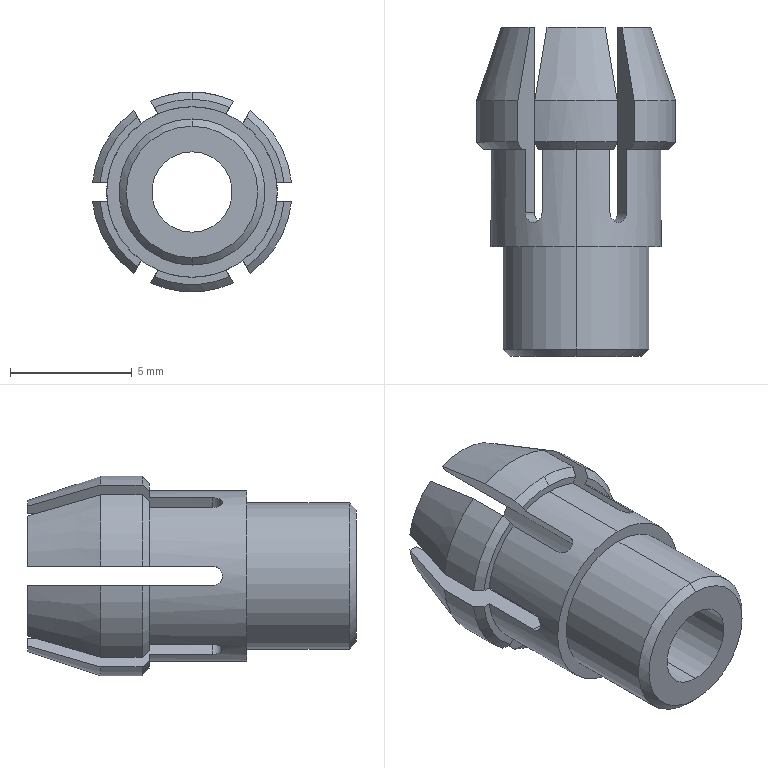Part | STEP file | 8mm elastic locating pin | 1 solid | 75 faces | box 8.161 x 13.5 x 8.2 mm | volume 235.099 mm3 | cylinder 32 | plane 27 | cone 16 | commonest cylinder face diameters 0.8 x12 5.5 x7 8.2 x7 3.3 x2 6 x2 7 x2